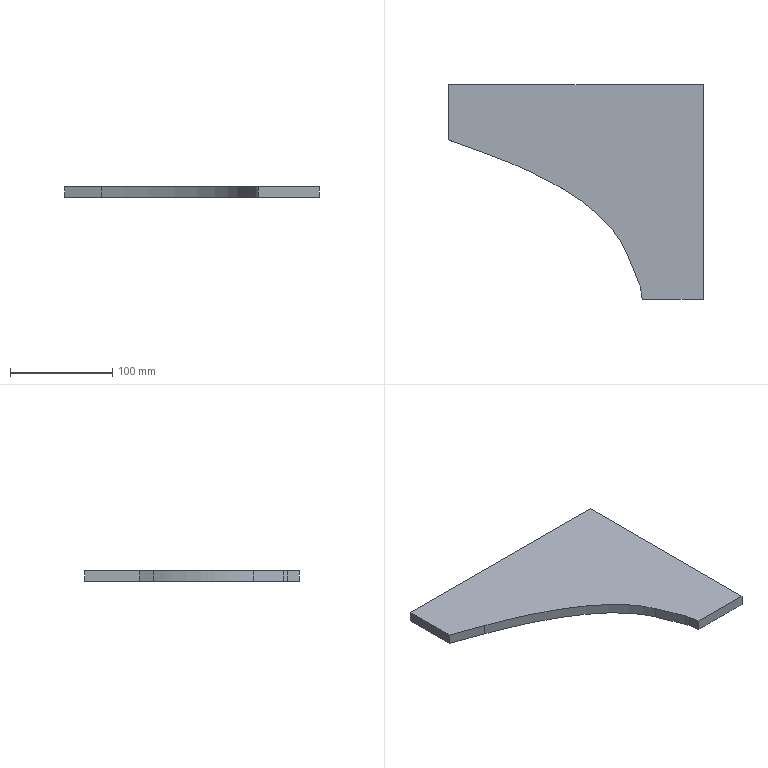Part | STEP file | 001-004-Feeding mechanism shaft entry channel base plate | 1 solid | 11 faces | box 249 x 210 x 10 mm | volume 317210 mm3 | plane 9 | cylinder 1 | spline 1 | commonest cylinder face diameters 40 x1
STEP:
#1=CARTESIAN_POINT('',(0.,0.,0.));
#2=DIRECTION('',(0.,0.,1.));
#3=DIRECTION('',(1.,0.,0.));
#4=AXIS2_PLACEMENT_3D('',#1,#2,#3);
#5=CARTESIAN_POINT('',(-124.5,50.933,10.));
#6=VERTEX_POINT('',#5);
#7=CARTESIAN_POINT('',(-124.5,50.933,0.));
#8=VERTEX_POINT('',#7);
#9=CARTESIAN_POINT('',(-124.5,50.933,10.));
#10=DIRECTION('',(0.,0.,-1.));
#11=VECTOR('',#10,1.);
#12=LINE('',#9,#11);
#13=CARTESIAN_POINT('',(-124.5,-105.,10.));
#14=DIRECTION('',(1.,0.,0.));
#15=DIRECTION('',(0.,0.,-1.));
#16=AXIS2_PLACEMENT_3D('',#13,#14,#15);
#17=PLANE('',#16);
#18=CARTESIAN_POINT('',(0.,155.933));
#19=DIRECTION('',(1.,0.));
#20=VECTOR('',#19,1.);
#21=LINE('',#18,#20);
#22=(GEOMETRIC_REPRESENTATION_CONTEXT(2)PARAMETRIC_REPRESENTATION_CONTEXT()REPRESENTATION_CONTEXT('',''));
#23=DEFINITIONAL_REPRESENTATION('',(#21),#22);
#24=PCURVE('',#17,#23);
#25=CARTESIAN_POINT('',(-124.5,50.933,10.));
#26=DIRECTION('',(-0.342,-0.9397,0.));
#27=DIRECTION('',(0.9397,-0.342,0.));
#28=AXIS2_PLACEMENT_3D('',#25,#26,#27);
#29=PLANE('',#28);
#30=CARTESIAN_POINT('',(0.,0.));
#31=DIRECTION('',(0.,-1.));
#32=VECTOR('',#31,1.);
#33=LINE('',#30,#32);
#34=(GEOMETRIC_REPRESENTATION_CONTEXT(2)PARAMETRIC_REPRESENTATION_CONTEXT()REPRESENTATION_CONTEXT('',''));
#35=DEFINITIONAL_REPRESENTATION('',(#33),#34);
#36=PCURVE('',#29,#35);
#37=SURFACE_CURVE('',#12,(#24,#36),.PCURVE_S1.);
#38=EDGE_CURVE('',#6,#8,#37,.T.);
#39=ORIENTED_EDGE('',*,*,#38,.F.);
#40=CARTESIAN_POINT('',(-124.5,105.,10.));
#41=VERTEX_POINT('',#40);
#42=CARTESIAN_POINT('',(-124.5,-105.,10.));
#43=DIRECTION('',(0.,-1.,0.));
#44=VECTOR('',#43,1.);
#45=LINE('',#42,#44);
#46=CARTESIAN_POINT('',(0.,0.));
#47=DIRECTION('',(0.,-1.));
#48=VECTOR('',#47,1.);
#49=LINE('',#46,#48);
#50=(GEOMETRIC_REPRESENTATION_CONTEXT(2)PARAMETRIC_REPRESENTATION_CONTEXT()REPRESENTATION_CONTEXT('',''));
#51=DEFINITIONAL_REPRESENTATION('',(#49),#50);
#52=PCURVE('',#17,#51);
#53=CARTESIAN_POINT('',(0.,0.,10.));
#54=DIRECTION('',(0.,0.,-1.));
#55=DIRECTION('',(-1.,0.,0.));
#56=AXIS2_PLACEMENT_3D('',#53,#54,#55);
#57=PLANE('',#56);
#58=CARTESIAN_POINT('',(124.5,-105.));
#59=DIRECTION('',(0.,-1.));
#60=VECTOR('',#59,1.);
#61=LINE('',#58,#60);
#62=(GEOMETRIC_REPRESENTATION_CONTEXT(2)PARAMETRIC_REPRESENTATION_CONTEXT()REPRESENTATION_CONTEXT('',''));
#63=DEFINITIONAL_REPRESENTATION('',(#61),#62);
#64=PCURVE('',#57,#63);
#65=SURFACE_CURVE('',#45,(#52,#64),.PCURVE_S1.);
#66=EDGE_CURVE('',#41,#6,#65,.T.);
#67=ORIENTED_EDGE('',*,*,#66,.F.);
#68=CARTESIAN_POINT('',(-124.5,105.,0.));
#69=VERTEX_POINT('',#68);
#70=CARTESIAN_POINT('',(-124.5,105.,10.));
#71=DIRECTION('',(0.,0.,-1.));
#72=VECTOR('',#71,1.);
#73=LINE('',#70,#72);
#74=CARTESIAN_POINT('',(0.,210.));
#75=DIRECTION('',(1.,0.));
#76=VECTOR('',#75,1.);
#77=LINE('',#74,#76);
#78=(GEOMETRIC_REPRESENTATION_CONTEXT(2)PARAMETRIC_REPRESENTATION_CONTEXT()REPRESENTATION_CONTEXT('',''));
#79=DEFINITIONAL_REPRESENTATION('',(#77),#78);
#80=PCURVE('',#17,#79);
#81=CARTESIAN_POINT('',(-124.5,105.,10.));
#82=DIRECTION('',(0.,-1.,0.));
#83=DIRECTION('',(0.,0.,-1.));
#84=AXIS2_PLACEMENT_3D('',#81,#82,#83);
#85=PLANE('',#84);
#86=CARTESIAN_POINT('',(0.,0.));
#87=DIRECTION('',(1.,0.));
#88=VECTOR('',#87,1.);
#89=LINE('',#86,#88);
#90=(GEOMETRIC_REPRESENTATION_CONTEXT(2)PARAMETRIC_REPRESENTATION_CONTEXT()REPRESENTATION_CONTEXT('',''));
#91=DEFINITIONAL_REPRESENTATION('',(#89),#90);
#92=PCURVE('',#85,#91);
#93=SURFACE_CURVE('',#73,(#80,#92),.PCURVE_S1.);
#94=EDGE_CURVE('',#41,#69,#93,.T.);
#95=ORIENTED_EDGE('',*,*,#94,.T.);
#96=CARTESIAN_POINT('',(-124.5,-105.,0.));
#97=DIRECTION('',(0.,-1.,0.));
#98=VECTOR('',#97,1.);
#99=LINE('',#96,#98);
#100=CARTESIAN_POINT('',(10.,0.));
#101=DIRECTION('',(0.,-1.));
#102=VECTOR('',#101,1.);
#103=LINE('',#100,#102);
#104=(GEOMETRIC_REPRESENTATION_CONTEXT(2)PARAMETRIC_REPRESENTATION_CONTEXT()REPRESENTATION_CONTEXT('',''));
#105=DEFINITIONAL_REPRESENTATION('',(#103),#104);
#106=PCURVE('',#17,#105);
#107=CARTESIAN_POINT('',(0.,0.,0.));
#108=DIRECTION('',(0.,0.,-1.));
#109=DIRECTION('',(-1.,0.,0.));
#110=AXIS2_PLACEMENT_3D('',#107,#108,#109);
#111=PLANE('',#110);
#112=CARTESIAN_POINT('',(124.5,-105.));
#113=DIRECTION('',(0.,-1.));
#114=VECTOR('',#113,1.);
#115=LINE('',#112,#114);
#116=(GEOMETRIC_REPRESENTATION_CONTEXT(2)PARAMETRIC_REPRESENTATION_CONTEXT()REPRESENTATION_CONTEXT('',''));
#117=DEFINITIONAL_REPRESENTATION('',(#115),#116);
#118=PCURVE('',#111,#117);
#119=SURFACE_CURVE('',#99,(#106,#118),.PCURVE_S1.);
#120=EDGE_CURVE('',#69,#8,#119,.T.);
#121=ORIENTED_EDGE('',*,*,#120,.T.);
#122=EDGE_LOOP('',(#39,#67,#95,#121));
#123=FACE_BOUND('',#122,.T.);
#124=ADVANCED_FACE('',(#123),#17,.F.);
#125=CARTESIAN_POINT('',(64.883,-105.,10.));
#126=VERTEX_POINT('',#125);
#127=CARTESIAN_POINT('',(64.883,-105.,0.));
#128=VERTEX_POINT('',#127);
#129=CARTESIAN_POINT('',(64.883,-105.,10.));
#130=DIRECTION('',(0.,0.,-1.));
#131=VECTOR('',#130,1.);
#132=LINE('',#129,#131);
#133=CARTESIAN_POINT('',(-124.5,-105.,10.));
#134=DIRECTION('',(0.,1.,0.));
#135=DIRECTION('',(0.,0.,1.));
#136=AXIS2_PLACEMENT_3D('',#133,#134,#135);
#137=PLANE('',#136);
#138=CARTESIAN_POINT('',(0.,189.383));
#139=DIRECTION('',(-1.,0.));
#140=VECTOR('',#139,1.);
#141=LINE('',#138,#140);
#142=(GEOMETRIC_REPRESENTATION_CONTEXT(2)PARAMETRIC_REPRESENTATION_CONTEXT()REPRESENTATION_CONTEXT('',''));
#143=DEFINITIONAL_REPRESENTATION('',(#141),#142);
#144=PCURVE('',#137,#143);
#145=CARTESIAN_POINT('',(64.883,-105.,10.));
#146=DIRECTION('',(-0.9848,-0.1736,0.));
#147=DIRECTION('',(0.1736,-0.9848,0.));
#148=AXIS2_PLACEMENT_3D('',#145,#146,#147);
#149=PLANE('',#148);
#150=CARTESIAN_POINT('',(0.,0.));
#151=DIRECTION('',(0.,-1.));
#152=VECTOR('',#151,1.);
#153=LINE('',#150,#152);
#154=(GEOMETRIC_REPRESENTATION_CONTEXT(2)PARAMETRIC_REPRESENTATION_CONTEXT()REPRESENTATION_CONTEXT('',''));
#155=DEFINITIONAL_REPRESENTATION('',(#153),#154);
#156=PCURVE('',#149,#155);
#157=SURFACE_CURVE('',#132,(#144,#156),.PCURVE_S1.);
#158=EDGE_CURVE('',#126,#128,#157,.T.);
#159=ORIENTED_EDGE('',*,*,#158,.T.);
#160=CARTESIAN_POINT('',(124.5,-105.,0.));
#161=VERTEX_POINT('',#160);
#162=CARTESIAN_POINT('',(-124.5,-105.,0.));
#163=DIRECTION('',(1.,0.,0.));
#164=VECTOR('',#163,1.);
#165=LINE('',#162,#164);
#166=CARTESIAN_POINT('',(-10.,0.));
#167=DIRECTION('',(0.,1.));
#168=VECTOR('',#167,1.);
#169=LINE('',#166,#168);
#170=(GEOMETRIC_REPRESENTATION_CONTEXT(2)PARAMETRIC_REPRESENTATION_CONTEXT()REPRESENTATION_CONTEXT('',''));
#171=DEFINITIONAL_REPRESENTATION('',(#169),#170);
#172=PCURVE('',#137,#171);
#173=CARTESIAN_POINT('',(124.5,-105.));
#174=DIRECTION('',(-1.,0.));
#175=VECTOR('',#174,1.);
#176=LINE('',#173,#175);
#177=(GEOMETRIC_REPRESENTATION_CONTEXT(2)PARAMETRIC_REPRESENTATION_CONTEXT()REPRESENTATION_CONTEXT('',''));
#178=DEFINITIONAL_REPRESENTATION('',(#176),#177);
#179=PCURVE('',#111,#178);
#180=SURFACE_CURVE('',#165,(#172,#179),.PCURVE_S1.);
#181=EDGE_CURVE('',#128,#161,#180,.T.);
#182=ORIENTED_EDGE('',*,*,#181,.T.);
#183=CARTESIAN_POINT('',(124.5,-105.,10.));
#184=VERTEX_POINT('',#183);
#185=CARTESIAN_POINT('',(124.5,-105.,10.));
#186=DIRECTION('',(0.,0.,-1.));
#187=VECTOR('',#186,1.);
#188=LINE('',#185,#187);
#189=CARTESIAN_POINT('',(0.,249.));
#190=DIRECTION('',(-1.,0.));
#191=VECTOR('',#190,1.);
#192=LINE('',#189,#191);
#193=(GEOMETRIC_REPRESENTATION_CONTEXT(2)PARAMETRIC_REPRESENTATION_CONTEXT()REPRESENTATION_CONTEXT('',''));
#194=DEFINITIONAL_REPRESENTATION('',(#192),#193);
#195=PCURVE('',#137,#194);
#196=CARTESIAN_POINT('',(124.5,-105.,10.));
#197=DIRECTION('',(-1.,0.,0.));
#198=DIRECTION('',(0.,0.,1.));
#199=AXIS2_PLACEMENT_3D('',#196,#197,#198);
#200=PLANE('',#199);
#201=CARTESIAN_POINT('',(0.,0.));
#202=DIRECTION('',(-1.,0.));
#203=VECTOR('',#202,1.);
#204=LINE('',#201,#203);
#205=(GEOMETRIC_REPRESENTATION_CONTEXT(2)PARAMETRIC_REPRESENTATION_CONTEXT()REPRESENTATION_CONTEXT('',''));
#206=DEFINITIONAL_REPRESENTATION('',(#204),#205);
#207=PCURVE('',#200,#206);
#208=SURFACE_CURVE('',#188,(#195,#207),.PCURVE_S1.);
#209=EDGE_CURVE('',#184,#161,#208,.T.);
#210=ORIENTED_EDGE('',*,*,#209,.F.);
#211=CARTESIAN_POINT('',(-124.5,-105.,10.));
#212=DIRECTION('',(1.,0.,0.));
#213=VECTOR('',#212,1.);
#214=LINE('',#211,#213);
#215=CARTESIAN_POINT('',(0.,0.));
#216=DIRECTION('',(0.,1.));
#217=VECTOR('',#216,1.);
#218=LINE('',#215,#217);
#219=(GEOMETRIC_REPRESENTATION_CONTEXT(2)PARAMETRIC_REPRESENTATION_CONTEXT()REPRESENTATION_CONTEXT('',''));
#220=DEFINITIONAL_REPRESENTATION('',(#218),#219);
#221=PCURVE('',#137,#220);
#222=CARTESIAN_POINT('',(124.5,-105.));
#223=DIRECTION('',(-1.,0.));
#224=VECTOR('',#223,1.);
#225=LINE('',#222,#224);
#226=(GEOMETRIC_REPRESENTATION_CONTEXT(2)PARAMETRIC_REPRESENTATION_CONTEXT()REPRESENTATION_CONTEXT('',''));
#227=DEFINITIONAL_REPRESENTATION('',(#225),#226);
#228=PCURVE('',#57,#227);
#229=SURFACE_CURVE('',#214,(#221,#228),.PCURVE_S1.);
#230=EDGE_CURVE('',#126,#184,#229,.T.);
#231=ORIENTED_EDGE('',*,*,#230,.F.);
#232=EDGE_LOOP('',(#159,#182,#210,#231));
#233=FACE_BOUND('',#232,.T.);
#234=ADVANCED_FACE('',(#233),#137,.F.);
#235=CARTESIAN_POINT('',(62.862,-93.536,10.));
#236=VERTEX_POINT('',#235);
#237=CARTESIAN_POINT('',(64.883,-105.,10.));
#238=DIRECTION('',(-0.1736,0.9848,0.));
#239=VECTOR('',#238,1.);
#240=LINE('',#237,#239);
#241=CARTESIAN_POINT('',(-64.883,-105.));
#242=DIRECTION('',(0.1736,0.9848));
#243=VECTOR('',#242,1.);
#244=LINE('',#241,#243);
#245=(GEOMETRIC_REPRESENTATION_CONTEXT(2)PARAMETRIC_REPRESENTATION_CONTEXT()REPRESENTATION_CONTEXT('',''));
#246=DEFINITIONAL_REPRESENTATION('',(#244),#245);
#247=PCURVE('',#57,#246);
#248=CARTESIAN_POINT('',(0.,0.));
#249=DIRECTION('',(-1.,0.));
#250=VECTOR('',#249,1.);
#251=LINE('',#248,#250);
#252=(GEOMETRIC_REPRESENTATION_CONTEXT(2)PARAMETRIC_REPRESENTATION_CONTEXT()REPRESENTATION_CONTEXT('',''));
#253=DEFINITIONAL_REPRESENTATION('',(#251),#252);
#254=PCURVE('',#149,#253);
#255=SURFACE_CURVE('',#240,(#247,#254),.PCURVE_S1.);
#256=EDGE_CURVE('',#126,#236,#255,.T.);
#257=ORIENTED_EDGE('',*,*,#256,.F.);
#258=ORIENTED_EDGE('',*,*,#230,.T.);
#259=CARTESIAN_POINT('',(124.5,105.,10.));
#260=VERTEX_POINT('',#259);
#261=CARTESIAN_POINT('',(124.5,-105.,10.));
#262=DIRECTION('',(0.,1.,0.));
#263=VECTOR('',#262,1.);
#264=LINE('',#261,#263);
#265=CARTESIAN_POINT('',(-124.5,-105.));
#266=DIRECTION('',(0.,1.));
#267=VECTOR('',#266,1.);
#268=LINE('',#265,#267);
#269=(GEOMETRIC_REPRESENTATION_CONTEXT(2)PARAMETRIC_REPRESENTATION_CONTEXT()REPRESENTATION_CONTEXT('',''));
#270=DEFINITIONAL_REPRESENTATION('',(#268),#269);
#271=PCURVE('',#57,#270);
#272=CARTESIAN_POINT('',(0.,0.));
#273=DIRECTION('',(0.,1.));
#274=VECTOR('',#273,1.);
#275=LINE('',#272,#274);
#276=(GEOMETRIC_REPRESENTATION_CONTEXT(2)PARAMETRIC_REPRESENTATION_CONTEXT()REPRESENTATION_CONTEXT('',''));
#277=DEFINITIONAL_REPRESENTATION('',(#275),#276);
#278=PCURVE('',#200,#277);
#279=SURFACE_CURVE('',#264,(#271,#278),.PCURVE_S1.);
#280=EDGE_CURVE('',#184,#260,#279,.T.);
#281=ORIENTED_EDGE('',*,*,#280,.T.);
#282=CARTESIAN_POINT('',(-124.5,105.,10.));
#283=DIRECTION('',(-1.,0.,0.));
#284=VECTOR('',#283,1.);
#285=LINE('',#282,#284);
#286=CARTESIAN_POINT('',(124.5,105.));
#287=DIRECTION('',(1.,0.));
#288=VECTOR('',#287,1.);
#289=LINE('',#286,#288);
#290=(GEOMETRIC_REPRESENTATION_CONTEXT(2)PARAMETRIC_REPRESENTATION_CONTEXT()REPRESENTATION_CONTEXT('',''));
#291=DEFINITIONAL_REPRESENTATION('',(#289),#290);
#292=PCURVE('',#57,#291);
#293=CARTESIAN_POINT('',(0.,0.));
#294=DIRECTION('',(0.,-1.));
#295=VECTOR('',#294,1.);
#296=LINE('',#293,#295);
#297=(GEOMETRIC_REPRESENTATION_CONTEXT(2)PARAMETRIC_REPRESENTATION_CONTEXT()REPRESENTATION_CONTEXT('',''));
#298=DEFINITIONAL_REPRESENTATION('',(#296),#297);
#299=PCURVE('',#85,#298);
#300=SURFACE_CURVE('',#285,(#292,#299),.PCURVE_S1.);
#301=EDGE_CURVE('',#260,#41,#300,.T.);
#302=ORIENTED_EDGE('',*,*,#301,.T.);
#303=ORIENTED_EDGE('',*,*,#66,.T.);
#304=CARTESIAN_POINT('',(-88.181,37.714,10.));
#305=VERTEX_POINT('',#304);
#306=CARTESIAN_POINT('',(-124.5,50.933,10.));
#307=DIRECTION('',(-0.9397,0.342,0.));
#308=VECTOR('',#307,1.);
#309=LINE('',#306,#308);
#310=CARTESIAN_POINT('',(124.5,50.933));
#311=DIRECTION('',(0.9397,0.342));
#312=VECTOR('',#311,1.);
#313=LINE('',#310,#312);
#314=(GEOMETRIC_REPRESENTATION_CONTEXT(2)PARAMETRIC_REPRESENTATION_CONTEXT()REPRESENTATION_CONTEXT('',''));
#315=DEFINITIONAL_REPRESENTATION('',(#313),#314);
#316=PCURVE('',#57,#315);
#317=CARTESIAN_POINT('',(0.,0.));
#318=DIRECTION('',(-1.,0.));
#319=VECTOR('',#318,1.);
#320=LINE('',#317,#319);
#321=(GEOMETRIC_REPRESENTATION_CONTEXT(2)PARAMETRIC_REPRESENTATION_CONTEXT()REPRESENTATION_CONTEXT('',''));
#322=DEFINITIONAL_REPRESENTATION('',(#320),#321);
#323=PCURVE('',#29,#322);
#324=SURFACE_CURVE('',#309,(#316,#323),.PCURVE_S1.);
#325=EDGE_CURVE('',#305,#6,#324,.T.);
#326=ORIENTED_EDGE('',*,*,#325,.F.);
#327=CARTESIAN_POINT('',(49.777,-59.984,10.));
#328=VERTEX_POINT('',#327);
#329=CARTESIAN_POINT('',(49.777,-59.984,10.));
#330=CARTESIAN_POINT('',(49.375,-58.99,10.));
#331=CARTESIAN_POINT('',(48.537,-57.033,10.));
#332=CARTESIAN_POINT('',(46.646,-53.079,10.));
#333=CARTESIAN_POINT('',(43.895,-48.118,10.));
#334=CARTESIAN_POINT('',(39.912,-42.087,10.));
#335=CARTESIAN_POINT('',(33.622,-33.936,10.));
#336=CARTESIAN_POINT('',(23.804,-23.545,10.));
#337=CARTESIAN_POINT('',(8.622,-10.897,10.));
#338=CARTESIAN_POINT('',(-6.974,-0.3771,10.));
#339=CARTESIAN_POINT('',(-21.236,7.936,10.));
#340=CARTESIAN_POINT('',(-32.824,14.1,10.));
#341=CARTESIAN_POINT('',(-45.302,20.175,10.));
#342=CARTESIAN_POINT('',(-56.439,25.153,10.));
#343=CARTESIAN_POINT('',(-65.79,29.077,10.));
#344=CARTESIAN_POINT('',(-73.022,31.99,10.));
#345=CARTESIAN_POINT('',(-79.234,34.392,10.));
#346=CARTESIAN_POINT('',(-84.306,36.294,10.));
#347=CARTESIAN_POINT('',(-86.892,37.245,10.));
#348=CARTESIAN_POINT('',(-88.181,37.714,10.));
#349=B_SPLINE_CURVE_WITH_KNOTS('',3,(#329,#330,#331,#332,#333,#334,#335,#336,#337,#338,#339,#340,#341,#342,#343,#344,#345,#346,#347,#348),.UNSPECIFIED.,.F.,.F.,(4,1,1,1,1,1,1,1,1,1,1,1,1,1,1,1,1,4),(0.,0.03125,0.0625,0.125,0.1875,0.25,0.375,0.5,0.625,0.6875,0.75,0.8125,0.875,0.9062,0.9375,0.9688,0.9844,1.),.UNSPECIFIED.);
#350=CARTESIAN_POINT('',(-49.777,-59.984));
#351=CARTESIAN_POINT('',(-49.375,-58.99));
#352=CARTESIAN_POINT('',(-48.537,-57.033));
#353=CARTESIAN_POINT('',(-46.646,-53.079));
#354=CARTESIAN_POINT('',(-43.895,-48.118));
#355=CARTESIAN_POINT('',(-39.912,-42.087));
#356=CARTESIAN_POINT('',(-33.622,-33.936));
#357=CARTESIAN_POINT('',(-23.804,-23.545));
#358=CARTESIAN_POINT('',(-8.622,-10.897));
#359=CARTESIAN_POINT('',(6.974,-0.3771));
#360=CARTESIAN_POINT('',(21.236,7.936));
#361=CARTESIAN_POINT('',(32.824,14.1));
#362=CARTESIAN_POINT('',(45.302,20.175));
#363=CARTESIAN_POINT('',(56.439,25.153));
#364=CARTESIAN_POINT('',(65.79,29.077));
#365=CARTESIAN_POINT('',(73.022,31.99));
#366=CARTESIAN_POINT('',(79.234,34.392));
#367=CARTESIAN_POINT('',(84.306,36.294));
#368=CARTESIAN_POINT('',(86.892,37.245));
#369=CARTESIAN_POINT('',(88.181,37.714));
#370=B_SPLINE_CURVE_WITH_KNOTS('',3,(#350,#351,#352,#353,#354,#355,#356,#357,#358,#359,#360,#361,#362,#363,#364,#365,#366,#367,#368,#369),.UNSPECIFIED.,.F.,.F.,(4,1,1,1,1,1,1,1,1,1,1,1,1,1,1,1,1,4),(0.,0.03125,0.0625,0.125,0.1875,0.25,0.375,0.5,0.625,0.6875,0.75,0.8125,0.875,0.9062,0.9375,0.9688,0.9844,1.),.UNSPECIFIED.);
#371=(GEOMETRIC_REPRESENTATION_CONTEXT(2)PARAMETRIC_REPRESENTATION_CONTEXT()REPRESENTATION_CONTEXT('',''));
#372=DEFINITIONAL_REPRESENTATION('',(#370),#371);
#373=PCURVE('',#57,#372);
#374=CARTESIAN_POINT('',(49.777,-59.984,10.));
#375=CARTESIAN_POINT('',(49.777,-59.984,0.));
#376=CARTESIAN_POINT('',(49.375,-58.99,10.));
#377=CARTESIAN_POINT('',(49.375,-58.99,0.));
#378=CARTESIAN_POINT('',(48.537,-57.033,10.));
#379=CARTESIAN_POINT('',(48.537,-57.033,0.));
#380=CARTESIAN_POINT('',(46.646,-53.079,10.));
#381=CARTESIAN_POINT('',(46.646,-53.079,0.));
#382=CARTESIAN_POINT('',(43.895,-48.118,10.));
#383=CARTESIAN_POINT('',(43.895,-48.118,0.));
#384=CARTESIAN_POINT('',(39.912,-42.087,10.));
#385=CARTESIAN_POINT('',(39.912,-42.087,0.));
#386=CARTESIAN_POINT('',(33.622,-33.936,10.));
#387=CARTESIAN_POINT('',(33.622,-33.936,0.));
#388=CARTESIAN_POINT('',(23.804,-23.545,10.));
#389=CARTESIAN_POINT('',(23.804,-23.545,0.));
#390=CARTESIAN_POINT('',(8.622,-10.897,10.));
#391=CARTESIAN_POINT('',(8.622,-10.897,0.));
#392=CARTESIAN_POINT('',(-6.974,-0.3771,10.));
#393=CARTESIAN_POINT('',(-6.974,-0.3771,0.));
#394=CARTESIAN_POINT('',(-21.236,7.936,10.));
#395=CARTESIAN_POINT('',(-21.236,7.936,0.));
#396=CARTESIAN_POINT('',(-32.824,14.1,10.));
#397=CARTESIAN_POINT('',(-32.824,14.1,0.));
#398=CARTESIAN_POINT('',(-45.302,20.175,10.));
#399=CARTESIAN_POINT('',(-45.302,20.175,0.));
#400=CARTESIAN_POINT('',(-56.439,25.153,10.));
#401=CARTESIAN_POINT('',(-56.439,25.153,0.));
#402=CARTESIAN_POINT('',(-65.79,29.077,10.));
#403=CARTESIAN_POINT('',(-65.79,29.077,0.));
#404=CARTESIAN_POINT('',(-73.022,31.99,10.));
#405=CARTESIAN_POINT('',(-73.022,31.99,0.));
#406=CARTESIAN_POINT('',(-79.234,34.392,10.));
#407=CARTESIAN_POINT('',(-79.234,34.392,0.));
#408=CARTESIAN_POINT('',(-84.306,36.294,10.));
#409=CARTESIAN_POINT('',(-84.306,36.294,0.));
#410=CARTESIAN_POINT('',(-86.892,37.245,10.));
#411=CARTESIAN_POINT('',(-86.892,37.245,0.));
#412=CARTESIAN_POINT('',(-88.181,37.714,10.));
#413=CARTESIAN_POINT('',(-88.181,37.714,0.));
#414=B_SPLINE_SURFACE_WITH_KNOTS('',3,1,((#374,#375),(#376,#377),(#378,#379),(#380,#381),(#382,#383),(#384,#385),(#386,#387),(#388,#389),(#390,#391),(#392,#393),(#394,#395),(#396,#397),(#398,#399),(#400,#401),(#402,#403),(#404,#405),(#406,#407),(#408,#409),(#410,#411),(#412,#413)),.UNSPECIFIED.,.F.,.F.,.F.,(4,1,1,1,1,1,1,1,1,1,1,1,1,1,1,1,1,4),(2,2),(0.,0.03125,0.0625,0.125,0.1875,0.25,0.375,0.5,0.625,0.6875,0.75,0.8125,0.875,0.9062,0.9375,0.9688,0.9844,1.),(0.,1.),.UNSPECIFIED.);
#415=CARTESIAN_POINT('',(0.,0.));
#416=DIRECTION('',(1.,0.));
#417=VECTOR('',#416,1.);
#418=LINE('',#415,#417);
#419=(GEOMETRIC_REPRESENTATION_CONTEXT(2)PARAMETRIC_REPRESENTATION_CONTEXT()REPRESENTATION_CONTEXT('',''));
#420=DEFINITIONAL_REPRESENTATION('',(#418),#419);
#421=PCURVE('',#414,#420);
#422=SURFACE_CURVE('',#349,(#373,#421),.PCURVE_S1.);
#423=EDGE_CURVE('',#328,#305,#422,.T.);
#424=ORIENTED_EDGE('',*,*,#423,.F.);
#425=CARTESIAN_POINT('',(61.709,-89.517,10.));
#426=VERTEX_POINT('',#425);
#427=CARTESIAN_POINT('',(61.709,-89.517,10.));
#428=DIRECTION('',(-0.3746,0.9272,0.));
#429=VECTOR('',#428,1.);
#430=LINE('',#427,#429);
#431=CARTESIAN_POINT('',(-61.709,-89.517));
#432=DIRECTION('',(0.3746,0.9272));
#433=VECTOR('',#432,1.);
#434=LINE('',#431,#433);
#435=(GEOMETRIC_REPRESENTATION_CONTEXT(2)PARAMETRIC_REPRESENTATION_CONTEXT()REPRESENTATION_CONTEXT('',''));
#436=DEFINITIONAL_REPRESENTATION('',(#434),#435);
#437=PCURVE('',#57,#436);
#438=CARTESIAN_POINT('',(61.709,-89.517,10.));
#439=DIRECTION('',(-0.9272,-0.3746,0.));
#440=DIRECTION('',(0.3746,-0.9272,0.));
#441=AXIS2_PLACEMENT_3D('',#438,#439,#440);
#442=PLANE('',#441);
#443=CARTESIAN_POINT('',(0.,0.));
#444=DIRECTION('',(-1.,0.));
#445=VECTOR('',#444,1.);
#446=LINE('',#443,#445);
#447=(GEOMETRIC_REPRESENTATION_CONTEXT(2)PARAMETRIC_REPRESENTATION_CONTEXT()REPRESENTATION_CONTEXT('',''));
#448=DEFINITIONAL_REPRESENTATION('',(#446),#447);
#449=PCURVE('',#442,#448);
#450=SURFACE_CURVE('',#430,(#437,#449),.PCURVE_S1.);
#451=EDGE_CURVE('',#426,#328,#450,.T.);
#452=ORIENTED_EDGE('',*,*,#451,.F.);
#453=CARTESIAN_POINT('',(43.165,-97.009,10.));
#454=DIRECTION('',(0.,0.,1.));
#455=DIRECTION('',(-1.,0.,0.));
#456=AXIS2_PLACEMENT_3D('',#453,#454,#455);
#457=CIRCLE('',#456,20.);
#458=CARTESIAN_POINT('',(-23.165,-97.009));
#459=CARTESIAN_POINT('',(-23.165,-131.65));
#460=CARTESIAN_POINT('',(-53.165,-114.33));
#461=CARTESIAN_POINT('',(-83.165,-97.009));
#462=CARTESIAN_POINT('',(-53.165,-79.689));
#463=CARTESIAN_POINT('',(-23.165,-62.368));
#464=CARTESIAN_POINT('',(-23.165,-97.009));
#465=(BOUNDED_CURVE()B_SPLINE_CURVE(2,(#458,#459,#460,#461,#462,#463,#464),.UNSPECIFIED.,.T.,.F.)B_SPLINE_CURVE_WITH_KNOTS((1,2,2,2,2,1),(-2.094,0.,2.094,4.189,6.283,8.378),.UNSPECIFIED.)CURVE()GEOMETRIC_REPRESENTATION_ITEM()RATIONAL_B_SPLINE_CURVE((1.,0.5,1.,0.5,1.,0.5,1.))REPRESENTATION_ITEM(''));
#466=(GEOMETRIC_REPRESENTATION_CONTEXT(2)PARAMETRIC_REPRESENTATION_CONTEXT()REPRESENTATION_CONTEXT('',''));
#467=DEFINITIONAL_REPRESENTATION('',(#465),#466);
#468=PCURVE('',#57,#467);
#469=CARTESIAN_POINT('',(43.165,-97.009,10.));
#470=DIRECTION('',(0.,0.,-1.));
#471=DIRECTION('',(-1.,0.,0.));
#472=AXIS2_PLACEMENT_3D('',#469,#470,#471);
#473=CYLINDRICAL_SURFACE('',#472,20.);
#474=CARTESIAN_POINT('',(6.283,0.));
#475=DIRECTION('',(-1.,0.));
#476=VECTOR('',#475,1.);
#477=LINE('',#474,#476);
#478=(GEOMETRIC_REPRESENTATION_CONTEXT(2)PARAMETRIC_REPRESENTATION_CONTEXT()REPRESENTATION_CONTEXT('',''));
#479=DEFINITIONAL_REPRESENTATION('',(#477),#478);
#480=PCURVE('',#473,#479);
#481=SURFACE_CURVE('',#457,(#468,#480),.PCURVE_S1.);
#482=EDGE_CURVE('',#236,#426,#481,.T.);
#483=ORIENTED_EDGE('',*,*,#482,.F.);
#484=EDGE_LOOP('',(#257,#258,#281,#302,#303,#326,#424,#452,#483));
#485=FACE_BOUND('',#484,.T.);
#486=ADVANCED_FACE('',(#485),#57,.F.);
#487=ORIENTED_EDGE('',*,*,#181,.F.);
#488=CARTESIAN_POINT('',(62.862,-93.536,0.));
#489=VERTEX_POINT('',#488);
#490=CARTESIAN_POINT('',(64.883,-105.,0.));
#491=DIRECTION('',(-0.1736,0.9848,0.));
#492=VECTOR('',#491,1.);
#493=LINE('',#490,#492);
#494=CARTESIAN_POINT('',(-64.883,-105.));
#495=DIRECTION('',(0.1736,0.9848));
#496=VECTOR('',#495,1.);
#497=LINE('',#494,#496);
#498=(GEOMETRIC_REPRESENTATION_CONTEXT(2)PARAMETRIC_REPRESENTATION_CONTEXT()REPRESENTATION_CONTEXT('',''));
#499=DEFINITIONAL_REPRESENTATION('',(#497),#498);
#500=PCURVE('',#111,#499);
#501=CARTESIAN_POINT('',(0.,-10.));
#502=DIRECTION('',(-1.,0.));
#503=VECTOR('',#502,1.);
#504=LINE('',#501,#503);
#505=(GEOMETRIC_REPRESENTATION_CONTEXT(2)PARAMETRIC_REPRESENTATION_CONTEXT()REPRESENTATION_CONTEXT('',''));
#506=DEFINITIONAL_REPRESENTATION('',(#504),#505);
#507=PCURVE('',#149,#506);
#508=SURFACE_CURVE('',#493,(#500,#507),.PCURVE_S1.);
#509=EDGE_CURVE('',#128,#489,#508,.T.);
#510=ORIENTED_EDGE('',*,*,#509,.T.);
#511=CARTESIAN_POINT('',(61.709,-89.517,0.));
#512=VERTEX_POINT('',#511);
#513=CARTESIAN_POINT('',(43.165,-97.009,0.));
#514=DIRECTION('',(0.,0.,1.));
#515=DIRECTION('',(-1.,0.,0.));
#516=AXIS2_PLACEMENT_3D('',#513,#514,#515);
#517=CIRCLE('',#516,20.);
#518=CARTESIAN_POINT('',(-23.165,-97.009));
#519=CARTESIAN_POINT('',(-23.165,-131.65));
#520=CARTESIAN_POINT('',(-53.165,-114.33));
#521=CARTESIAN_POINT('',(-83.165,-97.009));
#522=CARTESIAN_POINT('',(-53.165,-79.689));
#523=CARTESIAN_POINT('',(-23.165,-62.368));
#524=CARTESIAN_POINT('',(-23.165,-97.009));
#525=(BOUNDED_CURVE()B_SPLINE_CURVE(2,(#518,#519,#520,#521,#522,#523,#524),.UNSPECIFIED.,.T.,.F.)B_SPLINE_CURVE_WITH_KNOTS((1,2,2,2,2,1),(-2.094,0.,2.094,4.189,6.283,8.378),.UNSPECIFIED.)CURVE()GEOMETRIC_REPRESENTATION_ITEM()RATIONAL_B_SPLINE_CURVE((1.,0.5,1.,0.5,1.,0.5,1.))REPRESENTATION_ITEM(''));
#526=(GEOMETRIC_REPRESENTATION_CONTEXT(2)PARAMETRIC_REPRESENTATION_CONTEXT()REPRESENTATION_CONTEXT('',''));
#527=DEFINITIONAL_REPRESENTATION('',(#525),#526);
#528=PCURVE('',#111,#527);
#529=CARTESIAN_POINT('',(6.283,10.));
#530=DIRECTION('',(-1.,0.));
#531=VECTOR('',#530,1.);
#532=LINE('',#529,#531);
#533=(GEOMETRIC_REPRESENTATION_CONTEXT(2)PARAMETRIC_REPRESENTATION_CONTEXT()REPRESENTATION_CONTEXT('',''));
#534=DEFINITIONAL_REPRESENTATION('',(#532),#533);
#535=PCURVE('',#473,#534);
#536=SURFACE_CURVE('',#517,(#528,#535),.PCURVE_S1.);
#537=EDGE_CURVE('',#489,#512,#536,.T.);
#538=ORIENTED_EDGE('',*,*,#537,.T.);
#539=CARTESIAN_POINT('',(49.777,-59.984,0.));
#540=VERTEX_POINT('',#539);
#541=CARTESIAN_POINT('',(61.709,-89.517,0.));
#542=DIRECTION('',(-0.3746,0.9272,0.));
#543=VECTOR('',#542,1.);
#544=LINE('',#541,#543);
#545=CARTESIAN_POINT('',(-61.709,-89.517));
#546=DIRECTION('',(0.3746,0.9272));
#547=VECTOR('',#546,1.);
#548=LINE('',#545,#547);
#549=(GEOMETRIC_REPRESENTATION_CONTEXT(2)PARAMETRIC_REPRESENTATION_CONTEXT()REPRESENTATION_CONTEXT('',''));
#550=DEFINITIONAL_REPRESENTATION('',(#548),#549);
#551=PCURVE('',#111,#550);
#552=CARTESIAN_POINT('',(0.,-10.));
#553=DIRECTION('',(-1.,0.));
#554=VECTOR('',#553,1.);
#555=LINE('',#552,#554);
#556=(GEOMETRIC_REPRESENTATION_CONTEXT(2)PARAMETRIC_REPRESENTATION_CONTEXT()REPRESENTATION_CONTEXT('',''));
#557=DEFINITIONAL_REPRESENTATION('',(#555),#556);
#558=PCURVE('',#442,#557);
#559=SURFACE_CURVE('',#544,(#551,#558),.PCURVE_S1.);
#560=EDGE_CURVE('',#512,#540,#559,.T.);
#561=ORIENTED_EDGE('',*,*,#560,.T.);
#562=CARTESIAN_POINT('',(-88.181,37.714,0.));
#563=VERTEX_POINT('',#562);
#564=CARTESIAN_POINT('',(49.777,-59.984,0.));
#565=CARTESIAN_POINT('',(49.375,-58.99,0.));
#566=CARTESIAN_POINT('',(48.537,-57.033,0.));
#567=CARTESIAN_POINT('',(46.646,-53.079,0.));
#568=CARTESIAN_POINT('',(43.895,-48.118,0.));
#569=CARTESIAN_POINT('',(39.912,-42.087,0.));
#570=CARTESIAN_POINT('',(33.622,-33.936,0.));
#571=CARTESIAN_POINT('',(23.804,-23.545,0.));
#572=CARTESIAN_POINT('',(8.622,-10.897,0.));
#573=CARTESIAN_POINT('',(-6.974,-0.3771,0.));
#574=CARTESIAN_POINT('',(-21.236,7.936,0.));
#575=CARTESIAN_POINT('',(-32.824,14.1,0.));
#576=CARTESIAN_POINT('',(-45.302,20.175,0.));
#577=CARTESIAN_POINT('',(-56.439,25.153,0.));
#578=CARTESIAN_POINT('',(-65.79,29.077,0.));
#579=CARTESIAN_POINT('',(-73.022,31.99,0.));
#580=CARTESIAN_POINT('',(-79.234,34.392,0.));
#581=CARTESIAN_POINT('',(-84.306,36.294,0.));
#582=CARTESIAN_POINT('',(-86.892,37.245,0.));
#583=CARTESIAN_POINT('',(-88.181,37.714,0.));
#584=B_SPLINE_CURVE_WITH_KNOTS('',3,(#564,#565,#566,#567,#568,#569,#570,#571,#572,#573,#574,#575,#576,#577,#578,#579,#580,#581,#582,#583),.UNSPECIFIED.,.F.,.F.,(4,1,1,1,1,1,1,1,1,1,1,1,1,1,1,1,1,4),(0.,0.03125,0.0625,0.125,0.1875,0.25,0.375,0.5,0.625,0.6875,0.75,0.8125,0.875,0.9062,0.9375,0.9688,0.9844,1.),.UNSPECIFIED.);
#585=CARTESIAN_POINT('',(-49.777,-59.984));
#586=CARTESIAN_POINT('',(-49.375,-58.99));
#587=CARTESIAN_POINT('',(-48.537,-57.033));
#588=CARTESIAN_POINT('',(-46.646,-53.079));
#589=CARTESIAN_POINT('',(-43.895,-48.118));
#590=CARTESIAN_POINT('',(-39.912,-42.087));
#591=CARTESIAN_POINT('',(-33.622,-33.936));
#592=CARTESIAN_POINT('',(-23.804,-23.545));
#593=CARTESIAN_POINT('',(-8.622,-10.897));
#594=CARTESIAN_POINT('',(6.974,-0.3771));
#595=CARTESIAN_POINT('',(21.236,7.936));
#596=CARTESIAN_POINT('',(32.824,14.1));
#597=CARTESIAN_POINT('',(45.302,20.175));
#598=CARTESIAN_POINT('',(56.439,25.153));
#599=CARTESIAN_POINT('',(65.79,29.077));
#600=CARTESIAN_POINT('',(73.022,31.99));
#601=CARTESIAN_POINT('',(79.234,34.392));
#602=CARTESIAN_POINT('',(84.306,36.294));
#603=CARTESIAN_POINT('',(86.892,37.245));
#604=CARTESIAN_POINT('',(88.181,37.714));
#605=B_SPLINE_CURVE_WITH_KNOTS('',3,(#585,#586,#587,#588,#589,#590,#591,#592,#593,#594,#595,#596,#597,#598,#599,#600,#601,#602,#603,#604),.UNSPECIFIED.,.F.,.F.,(4,1,1,1,1,1,1,1,1,1,1,1,1,1,1,1,1,4),(0.,0.03125,0.0625,0.125,0.1875,0.25,0.375,0.5,0.625,0.6875,0.75,0.8125,0.875,0.9062,0.9375,0.9688,0.9844,1.),.UNSPECIFIED.);
#606=(GEOMETRIC_REPRESENTATION_CONTEXT(2)PARAMETRIC_REPRESENTATION_CONTEXT()REPRESENTATION_CONTEXT('',''));
#607=DEFINITIONAL_REPRESENTATION('',(#605),#606);
#608=PCURVE('',#111,#607);
#609=CARTESIAN_POINT('',(0.,1.));
#610=DIRECTION('',(1.,0.));
#611=VECTOR('',#610,1.);
#612=LINE('',#609,#611);
#613=(GEOMETRIC_REPRESENTATION_CONTEXT(2)PARAMETRIC_REPRESENTATION_CONTEXT()REPRESENTATION_CONTEXT('',''));
#614=DEFINITIONAL_REPRESENTATION('',(#612),#613);
#615=PCURVE('',#414,#614);
#616=SURFACE_CURVE('',#584,(#608,#615),.PCURVE_S1.);
#617=EDGE_CURVE('',#540,#563,#616,.T.);
#618=ORIENTED_EDGE('',*,*,#617,.T.);
#619=CARTESIAN_POINT('',(-124.5,50.933,0.));
#620=DIRECTION('',(-0.9397,0.342,0.));
#621=VECTOR('',#620,1.);
#622=LINE('',#619,#621);
#623=CARTESIAN_POINT('',(124.5,50.933));
#624=DIRECTION('',(0.9397,0.342));
#625=VECTOR('',#624,1.);
#626=LINE('',#623,#625);
#627=(GEOMETRIC_REPRESENTATION_CONTEXT(2)PARAMETRIC_REPRESENTATION_CONTEXT()REPRESENTATION_CONTEXT('',''));
#628=DEFINITIONAL_REPRESENTATION('',(#626),#627);
#629=PCURVE('',#111,#628);
#630=CARTESIAN_POINT('',(0.,-10.));
#631=DIRECTION('',(-1.,0.));
#632=VECTOR('',#631,1.);
#633=LINE('',#630,#632);
#634=(GEOMETRIC_REPRESENTATION_CONTEXT(2)PARAMETRIC_REPRESENTATION_CONTEXT()REPRESENTATION_CONTEXT('',''));
#635=DEFINITIONAL_REPRESENTATION('',(#633),#634);
#636=PCURVE('',#29,#635);
#637=SURFACE_CURVE('',#622,(#629,#636),.PCURVE_S1.);
#638=EDGE_CURVE('',#563,#8,#637,.T.);
#639=ORIENTED_EDGE('',*,*,#638,.T.);
#640=ORIENTED_EDGE('',*,*,#120,.F.);
#641=CARTESIAN_POINT('',(124.5,105.,0.));
#642=VERTEX_POINT('',#641);
#643=CARTESIAN_POINT('',(-124.5,105.,0.));
#644=DIRECTION('',(-1.,0.,0.));
#645=VECTOR('',#644,1.);
#646=LINE('',#643,#645);
#647=CARTESIAN_POINT('',(124.5,105.));
#648=DIRECTION('',(1.,0.));
#649=VECTOR('',#648,1.);
#650=LINE('',#647,#649);
#651=(GEOMETRIC_REPRESENTATION_CONTEXT(2)PARAMETRIC_REPRESENTATION_CONTEXT()REPRESENTATION_CONTEXT('',''));
#652=DEFINITIONAL_REPRESENTATION('',(#650),#651);
#653=PCURVE('',#111,#652);
#654=CARTESIAN_POINT('',(10.,0.));
#655=DIRECTION('',(0.,-1.));
#656=VECTOR('',#655,1.);
#657=LINE('',#654,#656);
#658=(GEOMETRIC_REPRESENTATION_CONTEXT(2)PARAMETRIC_REPRESENTATION_CONTEXT()REPRESENTATION_CONTEXT('',''));
#659=DEFINITIONAL_REPRESENTATION('',(#657),#658);
#660=PCURVE('',#85,#659);
#661=SURFACE_CURVE('',#646,(#653,#660),.PCURVE_S1.);
#662=EDGE_CURVE('',#642,#69,#661,.T.);
#663=ORIENTED_EDGE('',*,*,#662,.F.);
#664=CARTESIAN_POINT('',(124.5,-105.,0.));
#665=DIRECTION('',(0.,1.,0.));
#666=VECTOR('',#665,1.);
#667=LINE('',#664,#666);
#668=CARTESIAN_POINT('',(-124.5,-105.));
#669=DIRECTION('',(0.,1.));
#670=VECTOR('',#669,1.);
#671=LINE('',#668,#670);
#672=(GEOMETRIC_REPRESENTATION_CONTEXT(2)PARAMETRIC_REPRESENTATION_CONTEXT()REPRESENTATION_CONTEXT('',''));
#673=DEFINITIONAL_REPRESENTATION('',(#671),#672);
#674=PCURVE('',#111,#673);
#675=CARTESIAN_POINT('',(-10.,0.));
#676=DIRECTION('',(0.,1.));
#677=VECTOR('',#676,1.);
#678=LINE('',#675,#677);
#679=(GEOMETRIC_REPRESENTATION_CONTEXT(2)PARAMETRIC_REPRESENTATION_CONTEXT()REPRESENTATION_CONTEXT('',''));
#680=DEFINITIONAL_REPRESENTATION('',(#678),#679);
#681=PCURVE('',#200,#680);
#682=SURFACE_CURVE('',#667,(#674,#681),.PCURVE_S1.);
#683=EDGE_CURVE('',#161,#642,#682,.T.);
#684=ORIENTED_EDGE('',*,*,#683,.F.);
#685=EDGE_LOOP('',(#487,#510,#538,#561,#618,#639,#640,#663,#684));
#686=FACE_BOUND('',#685,.T.);
#687=ADVANCED_FACE('',(#686),#111,.T.);
#688=ORIENTED_EDGE('',*,*,#683,.T.);
#689=CARTESIAN_POINT('',(124.5,105.,10.));
#690=DIRECTION('',(0.,0.,-1.));
#691=VECTOR('',#690,1.);
#692=LINE('',#689,#691);
#693=CARTESIAN_POINT('',(0.,210.));
#694=DIRECTION('',(-1.,0.));
#695=VECTOR('',#694,1.);
#696=LINE('',#693,#695);
#697=(GEOMETRIC_REPRESENTATION_CONTEXT(2)PARAMETRIC_REPRESENTATION_CONTEXT()REPRESENTATION_CONTEXT('',''));
#698=DEFINITIONAL_REPRESENTATION('',(#696),#697);
#699=PCURVE('',#200,#698);
#700=CARTESIAN_POINT('',(0.,249.));
#701=DIRECTION('',(1.,0.));
#702=VECTOR('',#701,1.);
#703=LINE('',#700,#702);
#704=(GEOMETRIC_REPRESENTATION_CONTEXT(2)PARAMETRIC_REPRESENTATION_CONTEXT()REPRESENTATION_CONTEXT('',''));
#705=DEFINITIONAL_REPRESENTATION('',(#703),#704);
#706=PCURVE('',#85,#705);
#707=SURFACE_CURVE('',#692,(#699,#706),.PCURVE_S1.);
#708=EDGE_CURVE('',#260,#642,#707,.T.);
#709=ORIENTED_EDGE('',*,*,#708,.F.);
#710=ORIENTED_EDGE('',*,*,#280,.F.);
#711=ORIENTED_EDGE('',*,*,#209,.T.);
#712=EDGE_LOOP('',(#688,#709,#710,#711));
#713=FACE_BOUND('',#712,.T.);
#714=ADVANCED_FACE('',(#713),#200,.F.);
#715=ORIENTED_EDGE('',*,*,#662,.T.);
#716=ORIENTED_EDGE('',*,*,#94,.F.);
#717=ORIENTED_EDGE('',*,*,#301,.F.);
#718=ORIENTED_EDGE('',*,*,#708,.T.);
#719=EDGE_LOOP('',(#715,#716,#717,#718));
#720=FACE_BOUND('',#719,.T.);
#721=ADVANCED_FACE('',(#720),#85,.F.);
#722=ORIENTED_EDGE('',*,*,#509,.F.);
#723=ORIENTED_EDGE('',*,*,#158,.F.);
#724=ORIENTED_EDGE('',*,*,#256,.T.);
#725=CARTESIAN_POINT('',(62.862,-93.536,10.));
#726=DIRECTION('',(0.,0.,-1.));
#727=VECTOR('',#726,1.);
#728=LINE('',#725,#727);
#729=CARTESIAN_POINT('',(-11.641,0.));
#730=DIRECTION('',(0.,-1.));
#731=VECTOR('',#730,1.);
#732=LINE('',#729,#731);
#733=(GEOMETRIC_REPRESENTATION_CONTEXT(2)PARAMETRIC_REPRESENTATION_CONTEXT()REPRESENTATION_CONTEXT('',''));
#734=DEFINITIONAL_REPRESENTATION('',(#732),#733);
#735=PCURVE('',#149,#734);
#736=CARTESIAN_POINT('',(2.967,0.));
#737=DIRECTION('',(0.,1.));
#738=VECTOR('',#737,1.);
#739=LINE('',#736,#738);
#740=(GEOMETRIC_REPRESENTATION_CONTEXT(2)PARAMETRIC_REPRESENTATION_CONTEXT()REPRESENTATION_CONTEXT('',''));
#741=DEFINITIONAL_REPRESENTATION('',(#739),#740);
#742=PCURVE('',#473,#741);
#743=SURFACE_CURVE('',#728,(#735,#742),.PCURVE_S1.);
#744=EDGE_CURVE('',#236,#489,#743,.T.);
#745=ORIENTED_EDGE('',*,*,#744,.T.);
#746=EDGE_LOOP('',(#722,#723,#724,#745));
#747=FACE_BOUND('',#746,.T.);
#748=ADVANCED_FACE('',(#747),#149,.T.);
#749=CARTESIAN_POINT('',(61.709,-89.517,10.));
#750=DIRECTION('',(0.,0.,-1.));
#751=VECTOR('',#750,1.);
#752=LINE('',#749,#751);
#753=CARTESIAN_POINT('',(2.758,0.));
#754=DIRECTION('',(0.,1.));
#755=VECTOR('',#754,1.);
#756=LINE('',#753,#755);
#757=(GEOMETRIC_REPRESENTATION_CONTEXT(2)PARAMETRIC_REPRESENTATION_CONTEXT()REPRESENTATION_CONTEXT('',''));
#758=DEFINITIONAL_REPRESENTATION('',(#756),#757);
#759=PCURVE('',#473,#758);
#760=CARTESIAN_POINT('',(0.,0.));
#761=DIRECTION('',(0.,-1.));
#762=VECTOR('',#761,1.);
#763=LINE('',#760,#762);
#764=(GEOMETRIC_REPRESENTATION_CONTEXT(2)PARAMETRIC_REPRESENTATION_CONTEXT()REPRESENTATION_CONTEXT('',''));
#765=DEFINITIONAL_REPRESENTATION('',(#763),#764);
#766=PCURVE('',#442,#765);
#767=SURFACE_CURVE('',#752,(#759,#766),.PCURVE_S1.);
#768=EDGE_CURVE('',#426,#512,#767,.T.);
#769=ORIENTED_EDGE('',*,*,#768,.F.);
#770=ORIENTED_EDGE('',*,*,#482,.F.);
#771=ORIENTED_EDGE('',*,*,#744,.T.);
#772=ORIENTED_EDGE('',*,*,#537,.T.);
#773=EDGE_LOOP('',(#769,#770,#771,#772));
#774=FACE_BOUND('',#773,.F.);
#775=ADVANCED_FACE('',(#774),#473,.F.);
#776=ORIENTED_EDGE('',*,*,#560,.F.);
#777=ORIENTED_EDGE('',*,*,#768,.F.);
#778=ORIENTED_EDGE('',*,*,#451,.T.);
#779=CARTESIAN_POINT('',(49.777,-59.984,10.));
#780=DIRECTION('',(0.,0.,-1.));
#781=VECTOR('',#780,1.);
#782=LINE('',#779,#781);
#783=CARTESIAN_POINT('',(-31.852,0.));
#784=DIRECTION('',(0.,-1.));
#785=VECTOR('',#784,1.);
#786=LINE('',#783,#785);
#787=(GEOMETRIC_REPRESENTATION_CONTEXT(2)PARAMETRIC_REPRESENTATION_CONTEXT()REPRESENTATION_CONTEXT('',''));
#788=DEFINITIONAL_REPRESENTATION('',(#786),#787);
#789=PCURVE('',#442,#788);
#790=CARTESIAN_POINT('',(0.,0.));
#791=CARTESIAN_POINT('',(0.,1.));
#792=B_SPLINE_CURVE_WITH_KNOTS('',1,(#790,#791),.UNSPECIFIED.,.F.,.F.,(2,2),(0.,10.),.PIECEWISE_BEZIER_KNOTS.);
#793=(GEOMETRIC_REPRESENTATION_CONTEXT(2)PARAMETRIC_REPRESENTATION_CONTEXT()REPRESENTATION_CONTEXT('',''));
#794=DEFINITIONAL_REPRESENTATION('',(#792),#793);
#795=PCURVE('',#414,#794);
#796=SURFACE_CURVE('',#782,(#789,#795),.PCURVE_S1.);
#797=EDGE_CURVE('',#328,#540,#796,.T.);
#798=ORIENTED_EDGE('',*,*,#797,.T.);
#799=EDGE_LOOP('',(#776,#777,#778,#798));
#800=FACE_BOUND('',#799,.T.);
#801=ADVANCED_FACE('',(#800),#442,.T.);
#802=ORIENTED_EDGE('',*,*,#617,.F.);
#803=ORIENTED_EDGE('',*,*,#797,.F.);
#804=ORIENTED_EDGE('',*,*,#423,.T.);
#805=CARTESIAN_POINT('',(-88.181,37.714,10.));
#806=DIRECTION('',(0.,0.,-1.));
#807=VECTOR('',#806,1.);
#808=LINE('',#805,#807);
#809=CARTESIAN_POINT('',(1.,0.));
#810=CARTESIAN_POINT('',(1.,1.));
#811=B_SPLINE_CURVE_WITH_KNOTS('',1,(#809,#810),.UNSPECIFIED.,.F.,.F.,(2,2),(0.,10.),.PIECEWISE_BEZIER_KNOTS.);
#812=(GEOMETRIC_REPRESENTATION_CONTEXT(2)PARAMETRIC_REPRESENTATION_CONTEXT()REPRESENTATION_CONTEXT('',''));
#813=DEFINITIONAL_REPRESENTATION('',(#811),#812);
#814=PCURVE('',#414,#813);
#815=CARTESIAN_POINT('',(38.65,0.));
#816=DIRECTION('',(0.,-1.));
#817=VECTOR('',#816,1.);
#818=LINE('',#815,#817);
#819=(GEOMETRIC_REPRESENTATION_CONTEXT(2)PARAMETRIC_REPRESENTATION_CONTEXT()REPRESENTATION_CONTEXT('',''));
#820=DEFINITIONAL_REPRESENTATION('',(#818),#819);
#821=PCURVE('',#29,#820);
#822=SURFACE_CURVE('',#808,(#814,#821),.PCURVE_S1.);
#823=EDGE_CURVE('',#305,#563,#822,.T.);
#824=ORIENTED_EDGE('',*,*,#823,.T.);
#825=EDGE_LOOP('',(#802,#803,#804,#824));
#826=FACE_BOUND('',#825,.T.);
#827=ADVANCED_FACE('',(#826),#414,.T.);
#828=ORIENTED_EDGE('',*,*,#638,.F.);
#829=ORIENTED_EDGE('',*,*,#823,.F.);
#830=ORIENTED_EDGE('',*,*,#325,.T.);
#831=ORIENTED_EDGE('',*,*,#38,.T.);
#832=EDGE_LOOP('',(#828,#829,#830,#831));
#833=FACE_BOUND('',#832,.T.);
#834=ADVANCED_FACE('',(#833),#29,.T.);
#835=CLOSED_SHELL('',(#124,#234,#486,#687,#714,#721,#748,#775,#801,#827,#834));
#836=MANIFOLD_SOLID_BREP('',#835);
#837=(LENGTH_UNIT()NAMED_UNIT(*)SI_UNIT(.MILLI.,.METRE.));
#838=UNCERTAINTY_MEASURE_WITH_UNIT(LENGTH_MEASURE(0.0000001),#837,'','');
#839=(NAMED_UNIT(*)PLANE_ANGLE_UNIT()SI_UNIT($,.RADIAN.));
#840=(NAMED_UNIT(*)SI_UNIT($,.STERADIAN.)SOLID_ANGLE_UNIT());
#841=(GEOMETRIC_REPRESENTATION_CONTEXT(3)GLOBAL_UNCERTAINTY_ASSIGNED_CONTEXT((#838))GLOBAL_UNIT_ASSIGNED_CONTEXT((#837,#839,#840))REPRESENTATION_CONTEXT('',''));
#842=ADVANCED_BREP_SHAPE_REPRESENTATION('',(#4,#836),#841);